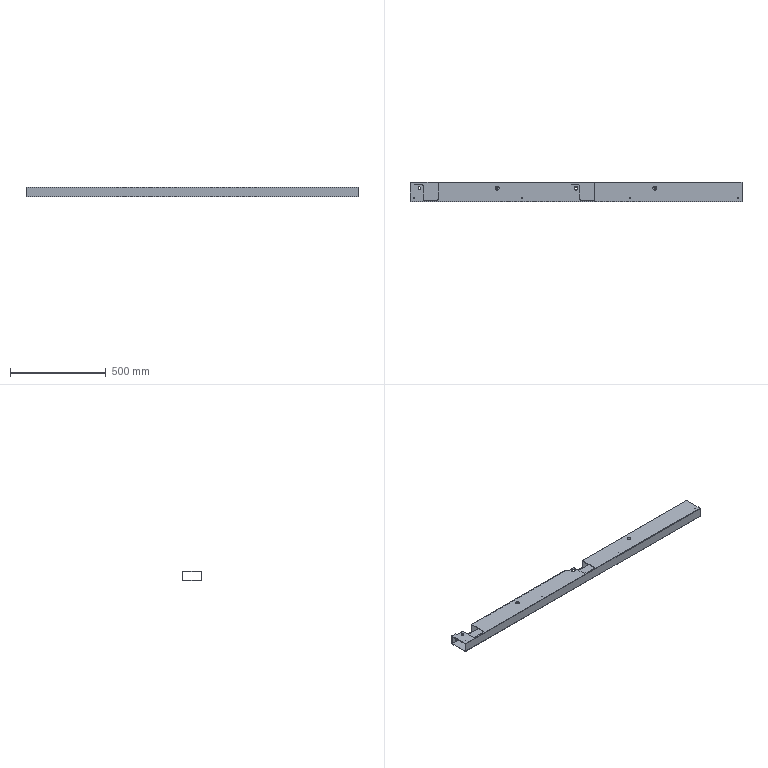Part | NX | features BREP 1 | 1 solid | 72 faces | box 1730 x 101.6 x 50.8 mm | volume 1433765 mm3 | cylinder 50 | plane 22 | commonest cylinder face diameters 3.81 x16 6.35 x10 3.175 x6 14.3 x6 8.128 x4 19.939 x4